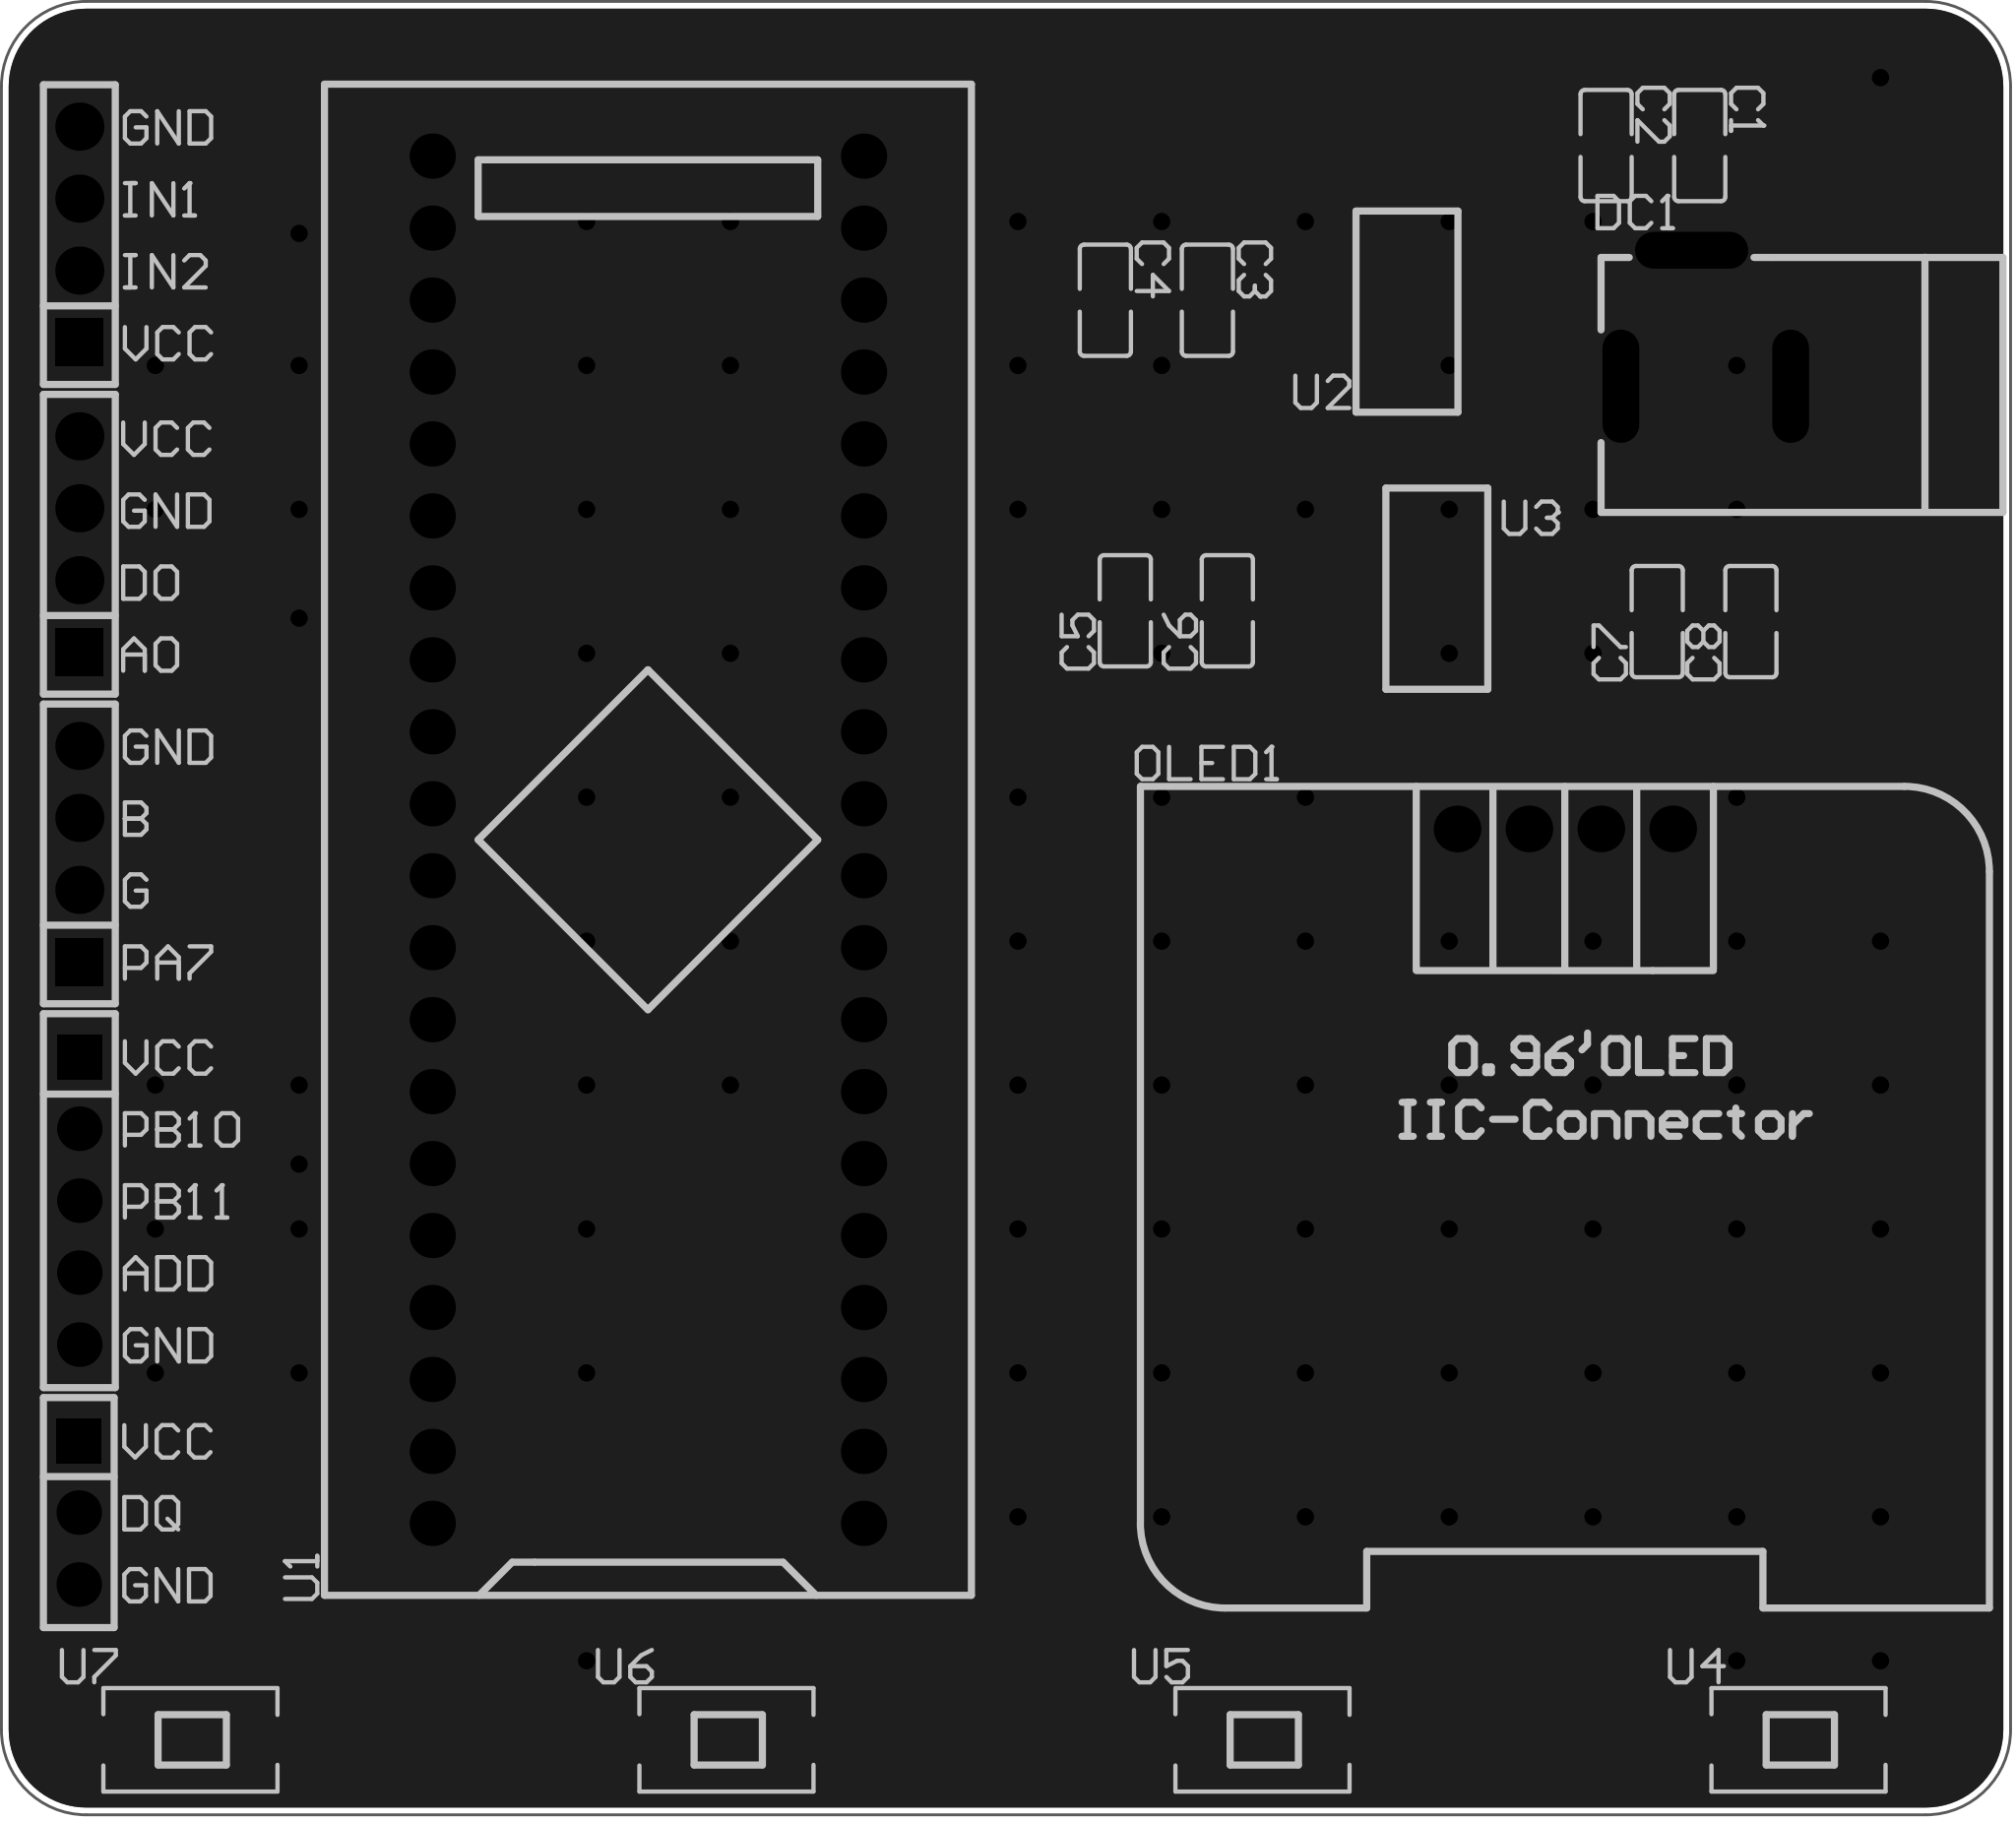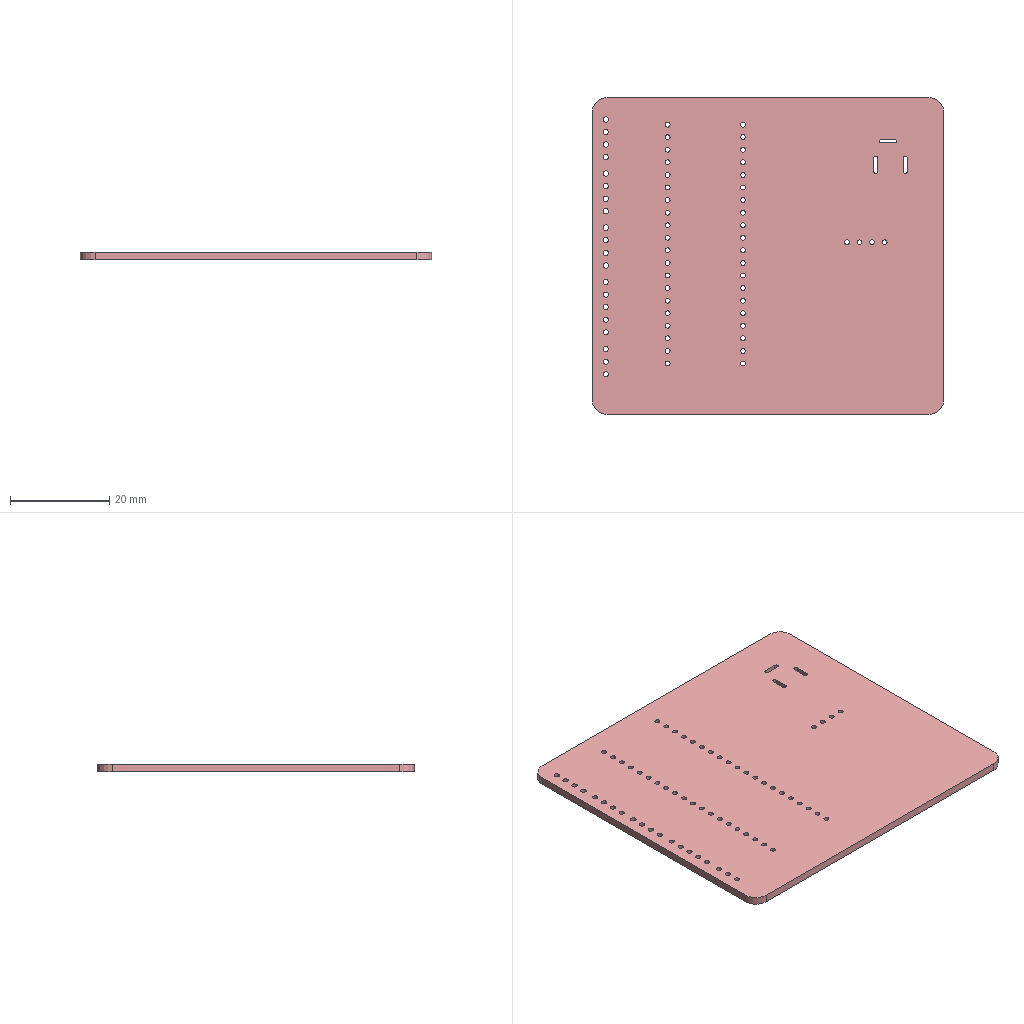Circuit board layout | Altium Designer | box 71 x 64 x 1.6 mm
Layer stack:
# Altium Designer layer stack of  (unit mm; dielectric type: 0 none, 1 core, 2 prepreg, 3 surface material)
index,name,kind,layer,copper_thickness_mm,dielectric_type,dielectric_thickness_mm,dielectric_material,dielectric_constant
0,Top Paste Mask Layer,other,,,,,,
1,Top Silkscreen Layer,other,,,,,,
2,Top Solder Mask Layer,dielectric,,,3,0.01,,3.3
3,Top Layer,copper,Top Layer,0.035,,,,
4,Dielectric1,dielectric,,,3,1.51,FR4,4.5
5,Bottom Layer,copper,Bottom Layer,0.035,,,,
6,Bottom Solder Mask Layer,dielectric,,,3,0.01,,3.3
7,Bottom Silkscreen Layer,other,,,,,,
8,Bottom Paste Mask Layer,other,,,,,,
# drill layer pairs: low layer,high layer
drill_pair,Top Layer,Bottom Layer
Part placement:
Designator,Comment,Layer,Footprint,Center-X(mm),Center-Y(mm),Rotation
C1,10uF,TopLayer,C0805,138.496,136.39,270
C2,100nF,TopLayer,C0805,135.187,136.39,270
C3,10uF,TopLayer,C0805,121.099,130.929,270
C4,100nF,TopLayer,C0805,117.493,130.929,270
C5,10uF,TopLayer,C0805,118.197,119.968,90
C6,100nF,TopLayer,C0805,121.803,119.968,90
C7,10uF,TopLayer,C0805,136.994,119.587,90
C8,100nF,TopLayer,C0805,140.303,119.587,90
DC1,,TopLayer,DC-2.0,138.709,130.294,0
H1,,TopLayer,HDR-TH_4P-P2.54-V-F,81.239,111.388,90
H2,,TopLayer,HDR-TH_5P-P2.54-V-F,81.239,99.148,270
H3,,TopLayer,HDR-TH_4P-P2.54-V-F,81.239,122.317,90
H4,,TopLayer,HDR-TH_3P-P2.54-V-F,81.219,88.138,270
H5,,TopLayer,HDR-TH_4P-P2.54-V-F,81.239,133.247,90
OLED1,,TopLayer,0.96OLED_4P,133.731,112.268,0
U1,STM32F103C8T6-Card,TopLayer,CONN-TH_L53.3-W22.9_STM32F103C8T6-CARD,101.331,111.887,90
U2,AMS1117-5.0,TopLayer,SOT_223,128.151,130.53,90
U3,AMS1117-3.3,TopLayer,SOT_223,129.207,120.748,270
U4,BX-TS-26-365TP,TopLayer,KEY-SMD_L6.0-W3.5-LS8.0-1,141.986,80.116,0
U5,BX-TS-26-365TP,TopLayer,KEY-SMD_L6.0-W3.5-LS8.0-1,123.045,80.116,0
U6,BX-TS-26-365TP,TopLayer,KEY-SMD_L6.0-W3.5-LS8.0-1,104.105,80.116,0
U7,BX-TS-26-365TP,TopLayer,KEY-SMD_L6.0-W3.5-LS8.0-1,85.164,80.116,0
Pad and via stacks:
# Altium Designer via and pad stacks of  (unit mm). Each distinct definition once, with the count of objects using it.
# via: kind,start_layer,end_layer,hole_mm,diameter_mm,mode(0 simple;1 top-mid-bottom;2 full stack),diameter_per_layer,count,example_net
# pad: kind,layer,hole_mm,hole_type(0 round;1 square;2 slot),plating,top_size,top_shape(1 round;2 rect;3 octagon;9 rounded rect),mid_size,bottom_size,mode,footprint,size_per_layer,count,example
pad,Top Layer,0,0,plated,1.41x1.35,2,1.41x1.35,1.41x1.35,0,C0805,,16,C1.2
pad,Top Layer,0,0,plated,2.2x3.5,2,2.2x3.5,2.2x3.5,0,SOT_223,,2,U2.4
pad,Top Layer,0,0,plated,1.1x2.2,2,1.1x2.2,1.1x2.2,0,SOT_223,,6,U2.3
pad,Top Layer,0,0,plated,1.74x1.4,2,1.74x1.4,1.74x1.4,0,KEY-SMD_L6.0-W3.5-LS8.0-1,,8,U4.1
pad,Multi-Layer,0.8001,2,plated,4x1.3,1,4x1.3,4x1.3,0,DC-2.0,,3,DC1.2
pad,Multi-Layer,1.1,0,plated,1.7x1.7,2,1.7x1.7,1.7x1.7,0,HDR-TH_4P-P2.54-V-F,,3,H1.1
pad,Multi-Layer,1.1,0,plated,1.7x1.7,1,1.7x1.7,1.7x1.7,0,HDR-TH_4P-P2.54-V-F,,9,H1.2
pad,Multi-Layer,1.02,0,plated,1.575x1.575,1,1.575x1.575,1.575x1.575,0,HDR-TH_5P-P2.54-V-F,,4,H2.5
pad,Multi-Layer,1.02,0,plated,1.575x1.575,2,1.575x1.575,1.575x1.575,0,HDR-TH_5P-P2.54-V-F,,1,H2.1
pad,Multi-Layer,1.02,0,plated,1.575x1.575,1,1.575x1.575,1.575x1.575,0,HDR-TH_3P-P2.54-V-F,,2,H4.3
pad,Multi-Layer,1.02,0,plated,1.575x1.575,2,1.575x1.575,1.575x1.575,0,HDR-TH_3P-P2.54-V-F,,1,H4.1
pad,Multi-Layer,1,0,plated,1.65x1.65,1,1.65x1.65,1.65x1.65,0,0.96OLED_4P,,4,OLED1.4
pad,Multi-Layer,1,0,plated,1.6x1.6,1,1.6x1.6,1.6x1.6,0,CONN-TH_L53.3-W22.9_STM32F103C8T6-CARD,,40,U1.1
via,Top Layer,Bottom Layer,0.3048,0.61,0,,90,GND
Copper pours:
name,layer,net,type(0 solid;1 hatched;2 none)
Top Layer-GND,Top Layer,GND,0
Bottom Layer-GND,Bottom Layer,GND,0